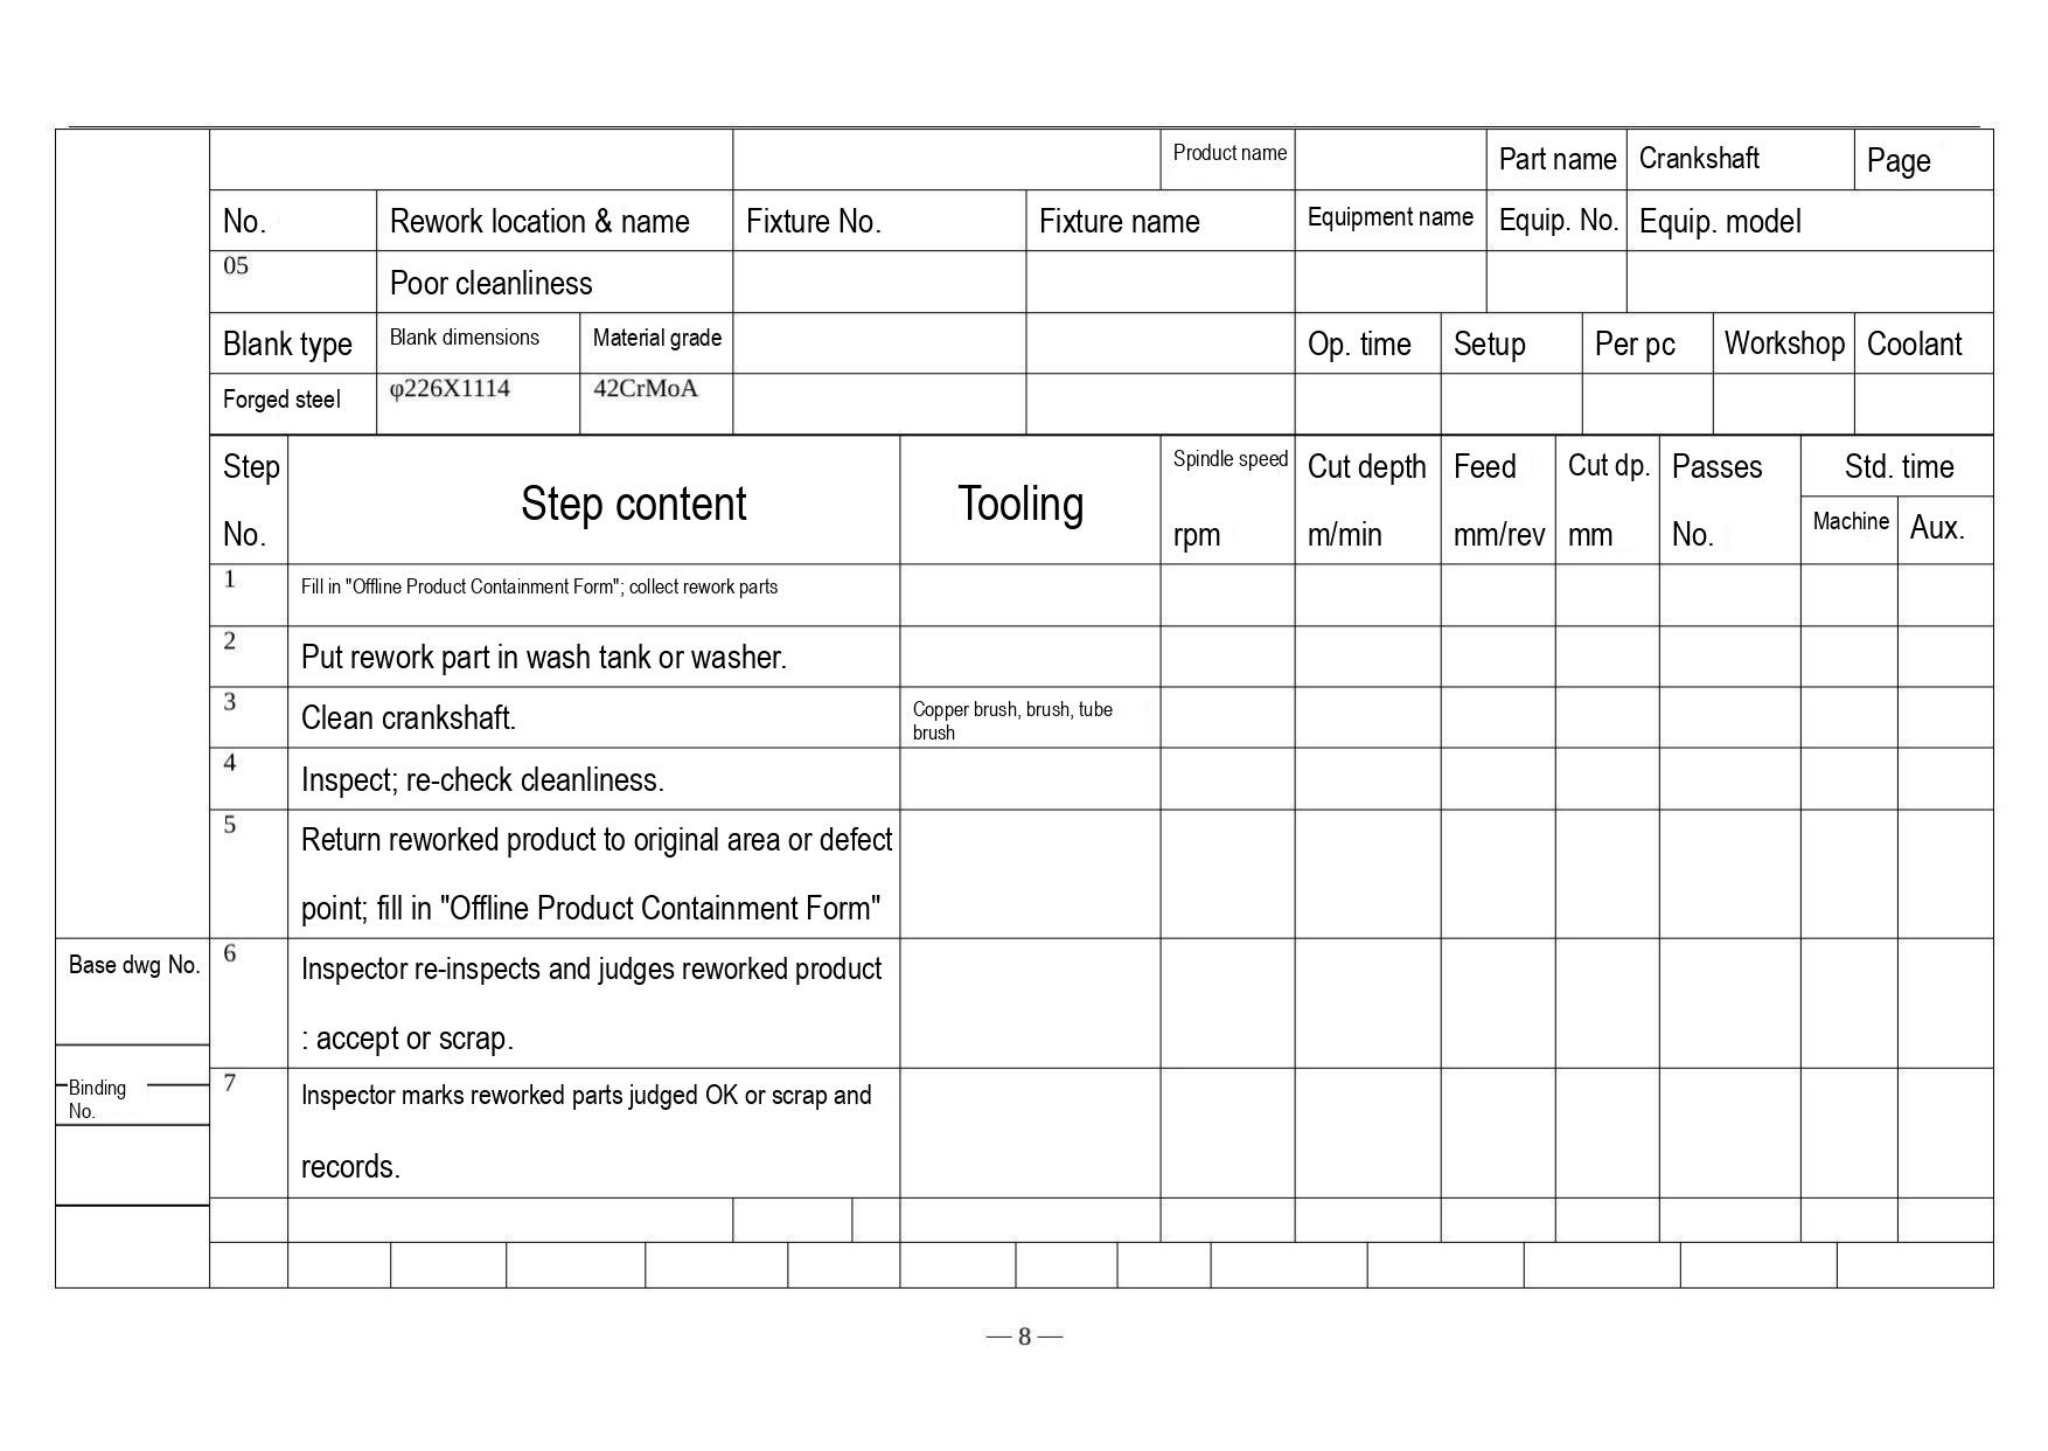| | | Product name | | Part name | Crankshaft | Page |
|---|---|---|---|---|---|---|

| No. | Rework location & name | Fixture No. | Fixture name | Equipment name | Equip. No. | Equip. model |
|---|---|---|---|---|---|---|
| 05 | Poor cleanliness | | | | | |

| Blank type | Blank dimensions | Material grade | | | Op. time | Setup | Per pc | Workshop | Coolant |
|---|---|---|---|---|---|---|---|---|---|
| Forged steel | φ226X1114 | 42CrMoA | | | | | | | |

| Step No. | Step content | Tooling | Spindle speed rpm | Cut depth m/min | Feed mm/rev | Cut dp. mm | Passes No. | Std. time Machine | Std. time Aux. |
|---|---|---|---|---|---|---|---|---|---|
| 1 | Fill in "Offline Product Containment Form"; collect rework parts | | | | | | | | |
| 2 | Put rework part in wash tank or washer. | | | | | | | | |
| 3 | Clean crankshaft. | Copper brush, brush, tube brush | | | | | | | |
| 4 | Inspect; re-check cleanliness. | | | | | | | | |
| 5 | Return reworked product to original area or defect point; fill in "Offline Product Containment Form" | | | | | | | | |
| 6 | Inspector re-inspects and judges reworked product : accept or scrap. | | | | | | | | |
| 7 | Inspector marks reworked parts judged OK or scrap and records. | | | | | | | | |

Base dwg No.

Binding No.

— 8 —
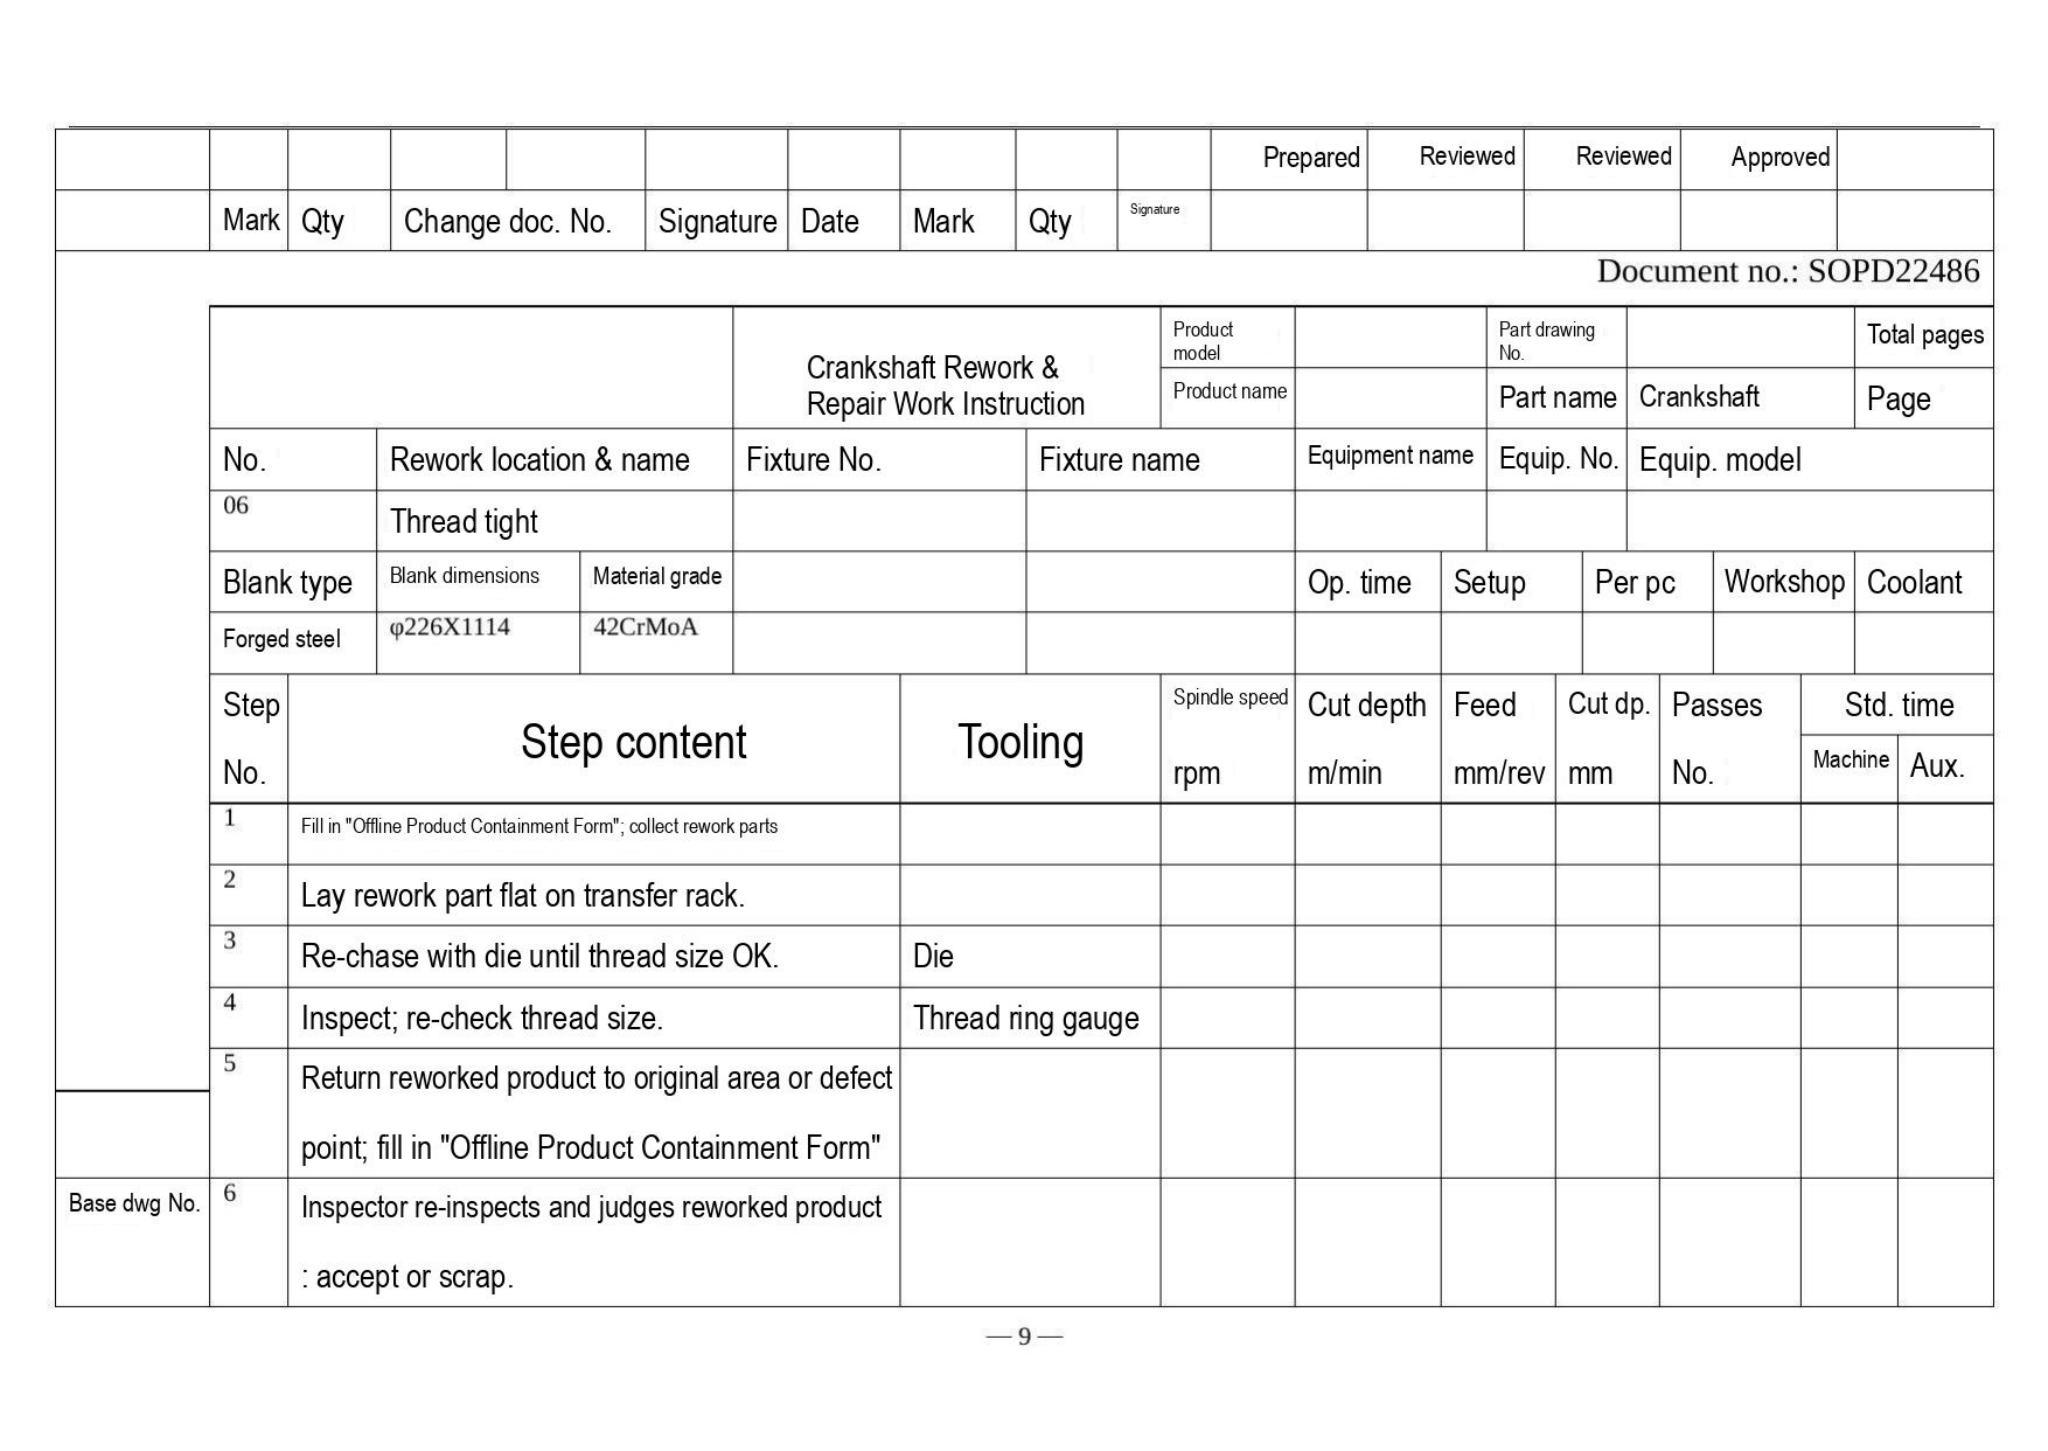Prepared | Reviewed | Reviewed | Approved

| Mark | Qty | Change doc. No. | Signature | Date | Mark | Qty | Signature |
|---|---|---|---|---|---|---|---|

Document no.: SOPD22486

| Crankshaft Rework & Repair Work Instruction | Product model | | Part drawing No. | | Total pages |
|---|---|---|---|---|---|
| | Product name | | Part name | Crankshaft | Page |

| No. | Rework location & name | Fixture No. | Fixture name | Equipment name | Equip. No. | Equip. model |
|---|---|---|---|---|---|---|
| 06 | Thread tight | | | | | |

| Blank type | Blank dimensions | Material grade | | | Op. time | Setup | Per pc | Workshop | Coolant |
|---|---|---|---|---|---|---|---|---|---|
| Forged steel | φ226X1114 | 42CrMoA | | | | | | | |

| Step No. | Step content | Tooling | Spindle speed rpm | Cut depth m/min | Feed mm/rev | Cut dp. mm | Passes No. | Std. time Machine | Std. time Aux. |
|---|---|---|---|---|---|---|---|---|---|
| 1 | Fill in "Offline Product Containment Form"; collect rework parts | | | | | | | | |
| 2 | Lay rework part flat on transfer rack. | | | | | | | | |
| 3 | Re-chase with die until thread size OK. | Die | | | | | | | |
| 4 | Inspect; re-check thread size. | Thread ring gauge | | | | | | | |
| 5 | Return reworked product to original area or defect point; fill in "Offline Product Containment Form" | | | | | | | | |
| 6 | Inspector re-inspects and judges reworked product : accept or scrap. | | | | | | | | |

Base dwg No.

— 9 —
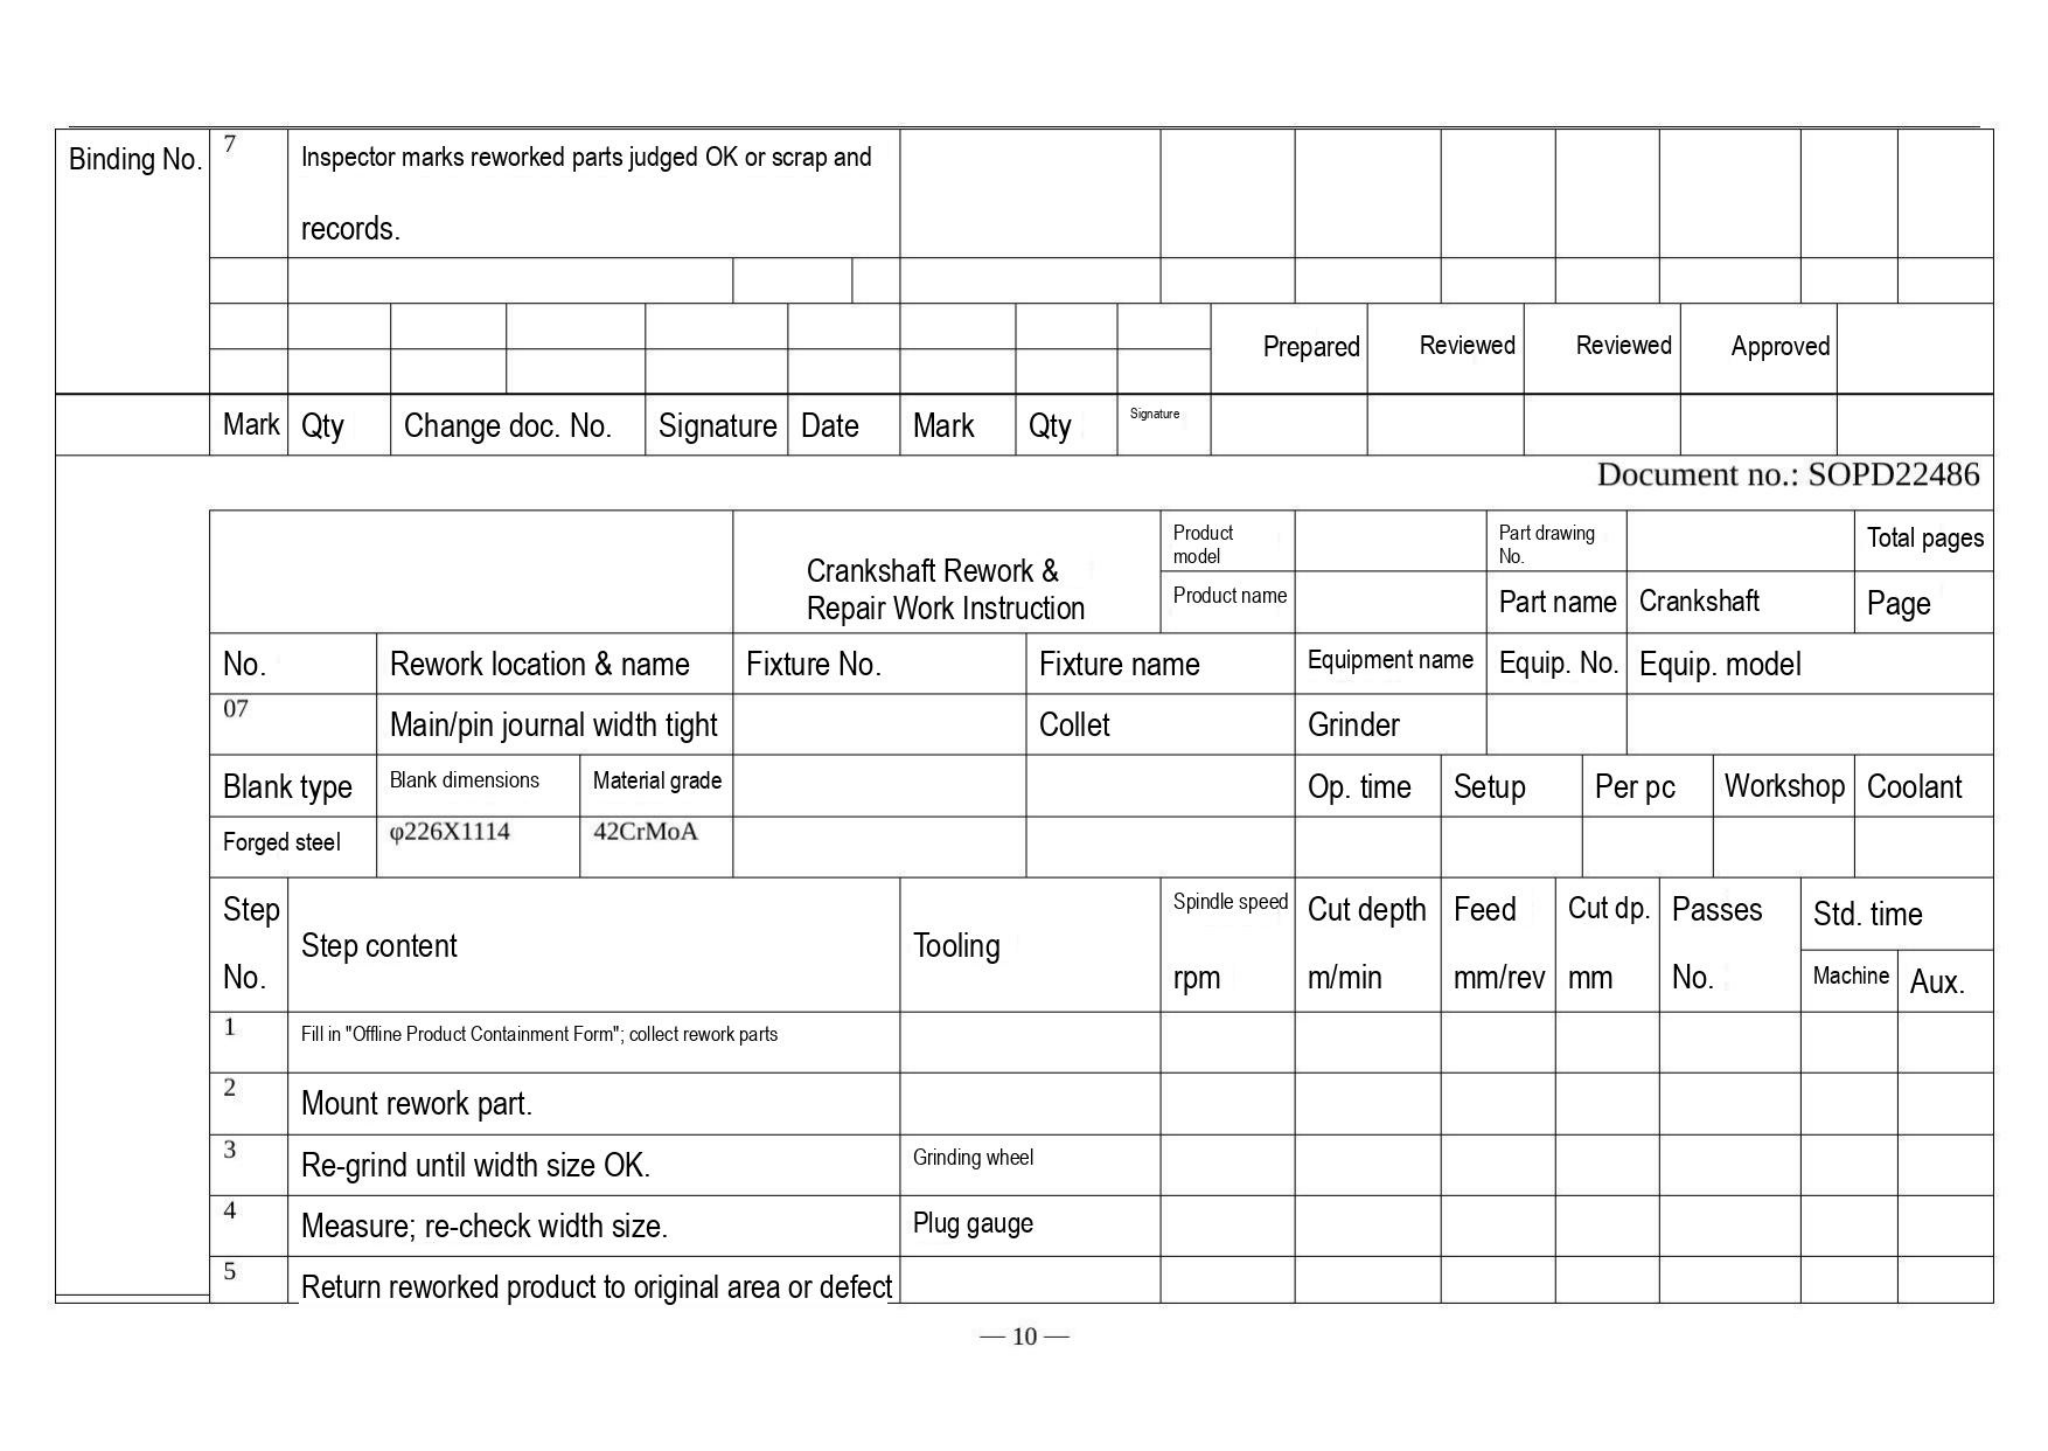| Binding No. | 7 | Inspector marks reworked parts judged OK or scrap and records. | | | | | | | |
|---|---|---|---|---|---|---|---|---|---|
| | | | | | | | | | |
| | | | | | | Prepared | Reviewed | Reviewed | Approved |
| | Mark | Qty | Change doc. No. | Signature | Date | Mark | Qty | Signature | |

Document no.: SOPD22486

| | Crankshaft Rework & Repair Work Instruction | Product model | | Part drawing No. | | Total pages |
|---|---|---|---|---|---|---|
| | | Product name | | Part name | Crankshaft | Page |

| No. | Rework location & name | Fixture No. | Fixture name | Equipment name | Equip. No. | Equip. model |
|---|---|---|---|---|---|---|
| 07 | Main/pin journal width tight | | Collet | Grinder | | |

| Blank type | Blank dimensions | Material grade | | | Op. time | Setup | Per pc | Workshop | Coolant |
|---|---|---|---|---|---|---|---|---|---|
| Forged steel | φ226X1114 | 42CrMoA | | | | | | | |

| Step No. | Step content | Tooling | Spindle speed rpm | Cut depth m/min | Feed mm/rev | Cut dp. mm | Passes No. | Std. time Machine | Std. time Aux. |
|---|---|---|---|---|---|---|---|---|---|
| 1 | Fill in "Offline Product Containment Form"; collect rework parts | | | | | | | | |
| 2 | Mount rework part. | | | | | | | | |
| 3 | Re-grind until width size OK. | Grinding wheel | | | | | | | |
| 4 | Measure; re-check width size. | Plug gauge | | | | | | | |
| 5 | Return reworked product to original area or defect | | | | | | | | |

— 10 —
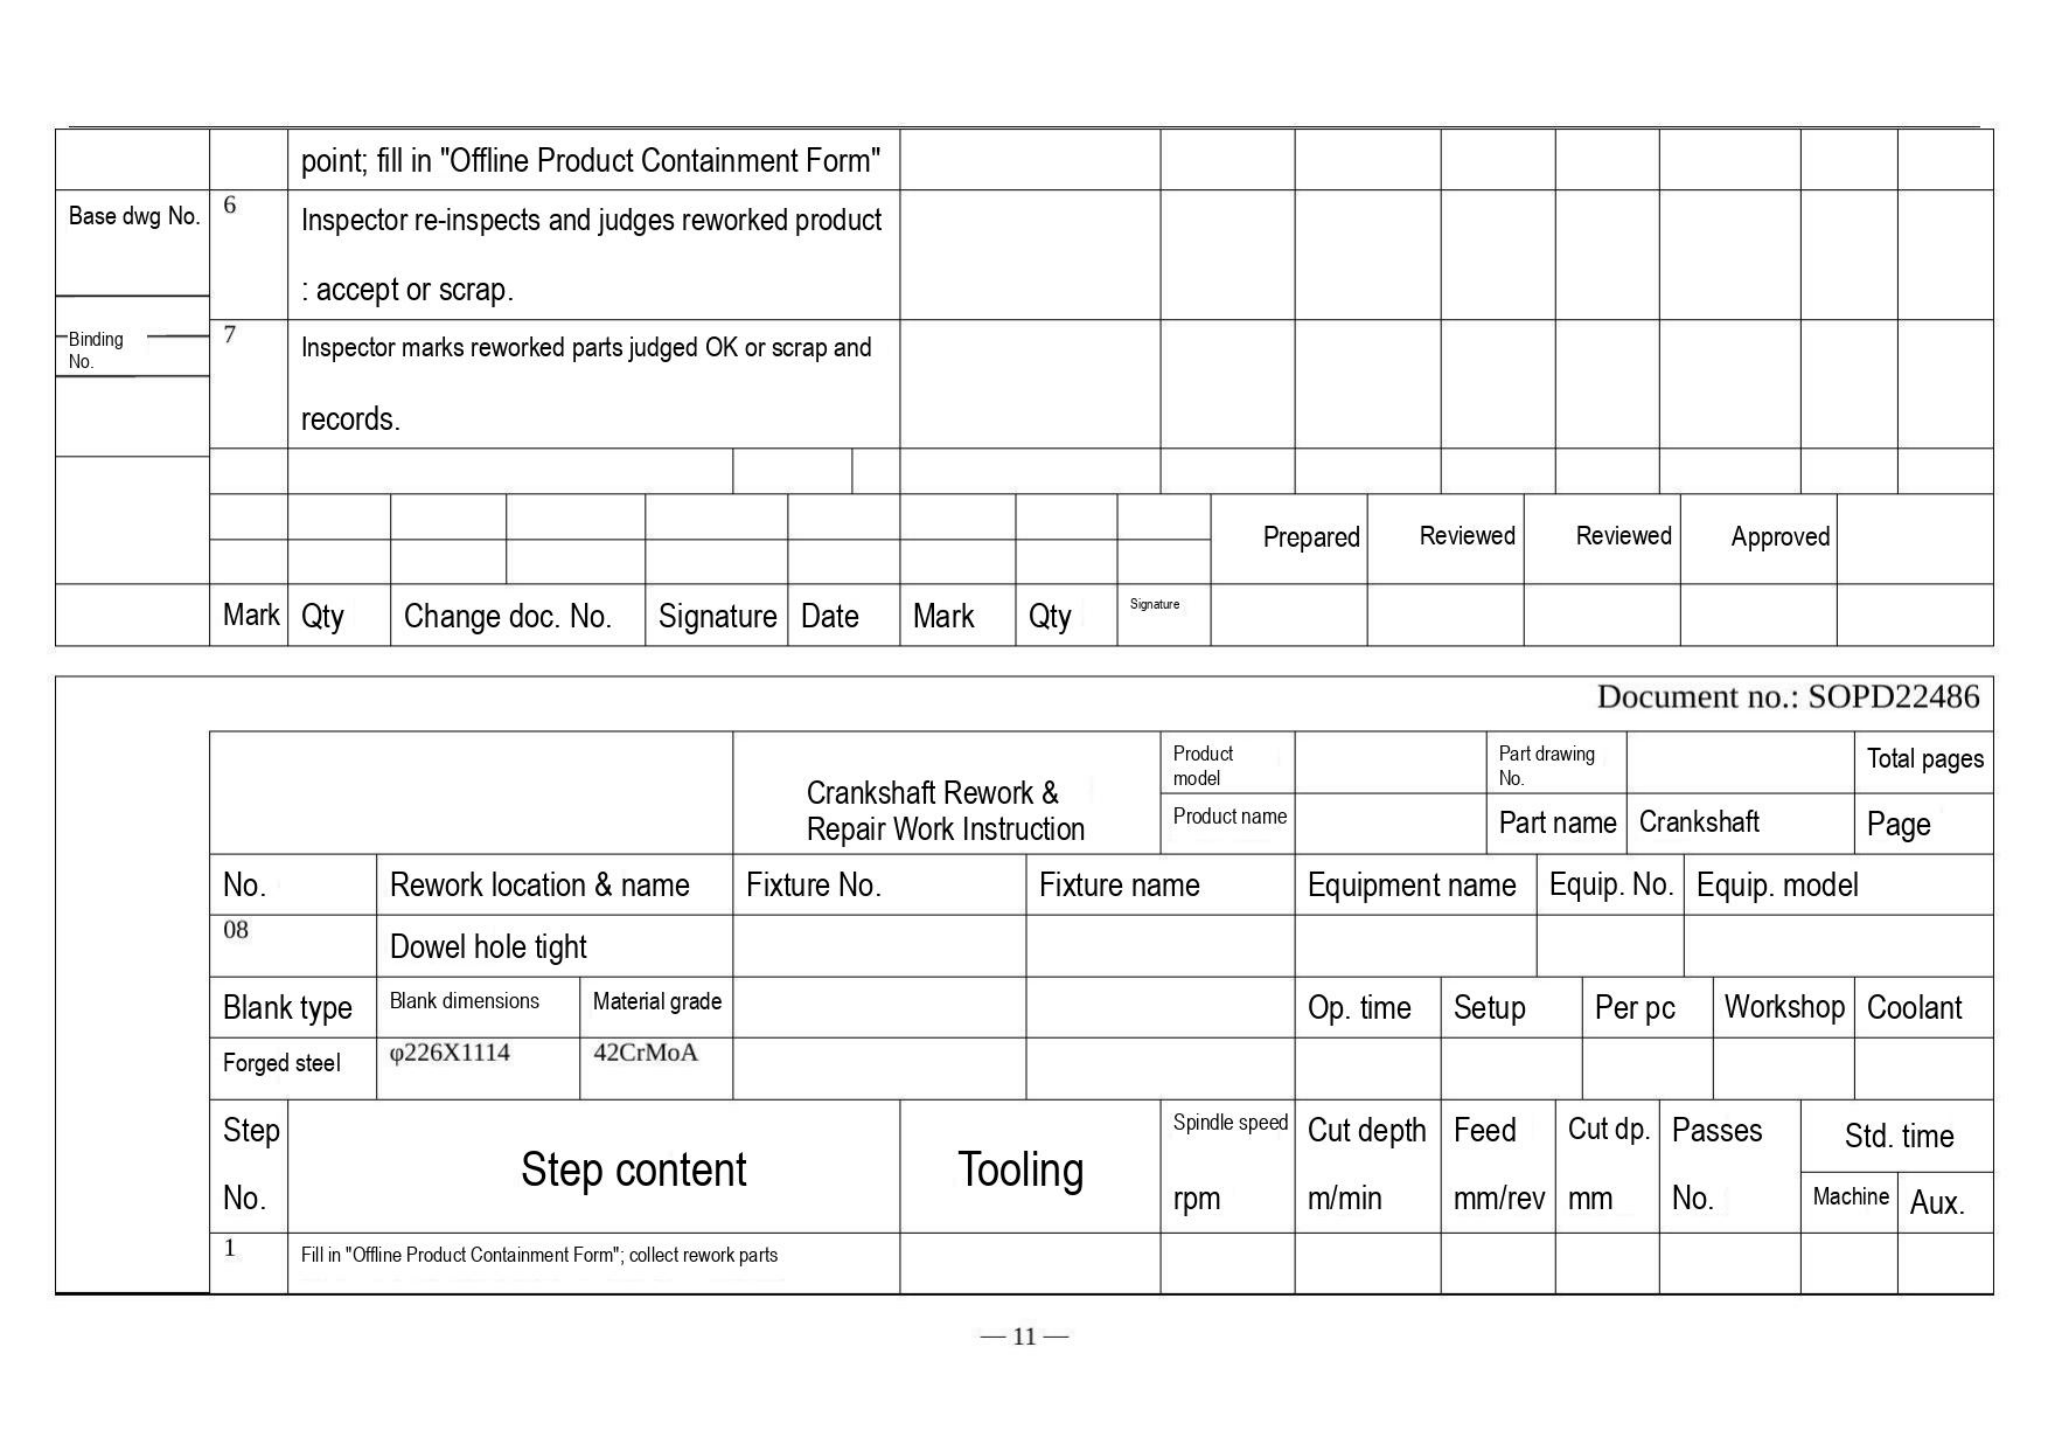| | | | | | | | | | | |
|---|---|---|---|---|---|---|---|---|---|---|
| | | point; fill in "Offline Product Containment Form" | | | | | | | | |
| Base dwg No. | 6 | Inspector re-inspects and judges reworked product : accept or scrap. | | | | | | | | |
| Binding No. | 7 | Inspector marks reworked parts judged OK or scrap and records. | | | | | | | | |

| | | | | | | | | Prepared | Reviewed | Reviewed | Approved | |
|---|---|---|---|---|---|---|---|---|---|---|---|---|
| Mark | Qty | Change doc. No. | Signature | Date | Mark | Qty | Signature | | | | | |

Document no.: SOPD22486

| | Crankshaft Rework & Repair Work Instruction | Product model | | Part drawing No. | | Total pages |
|---|---|---|---|---|---|---|
| | | Product name | | Part name | Crankshaft | Page |

| No. | Rework location & name | Fixture No. | Fixture name | Equipment name | Equip. No. | Equip. model |
|---|---|---|---|---|---|---|
| 08 | Dowel hole tight | | | | | |

| Blank type | Blank dimensions | Material grade | | | Op. time | Setup | Per pc | Workshop | Coolant |
|---|---|---|---|---|---|---|---|---|---|
| Forged steel | φ226X1114 | 42CrMoA | | | | | | | |

| Step No. | Step content | Tooling | Spindle speed rpm | Cut depth m/min | Feed mm/rev | Cut dp. mm | Passes No. | Std. time Machine | Std. time Aux. |
|---|---|---|---|---|---|---|---|---|---|
| 1 | Fill in "Offline Product Containment Form"; collect rework parts | | | | | | | | |

— 11 —
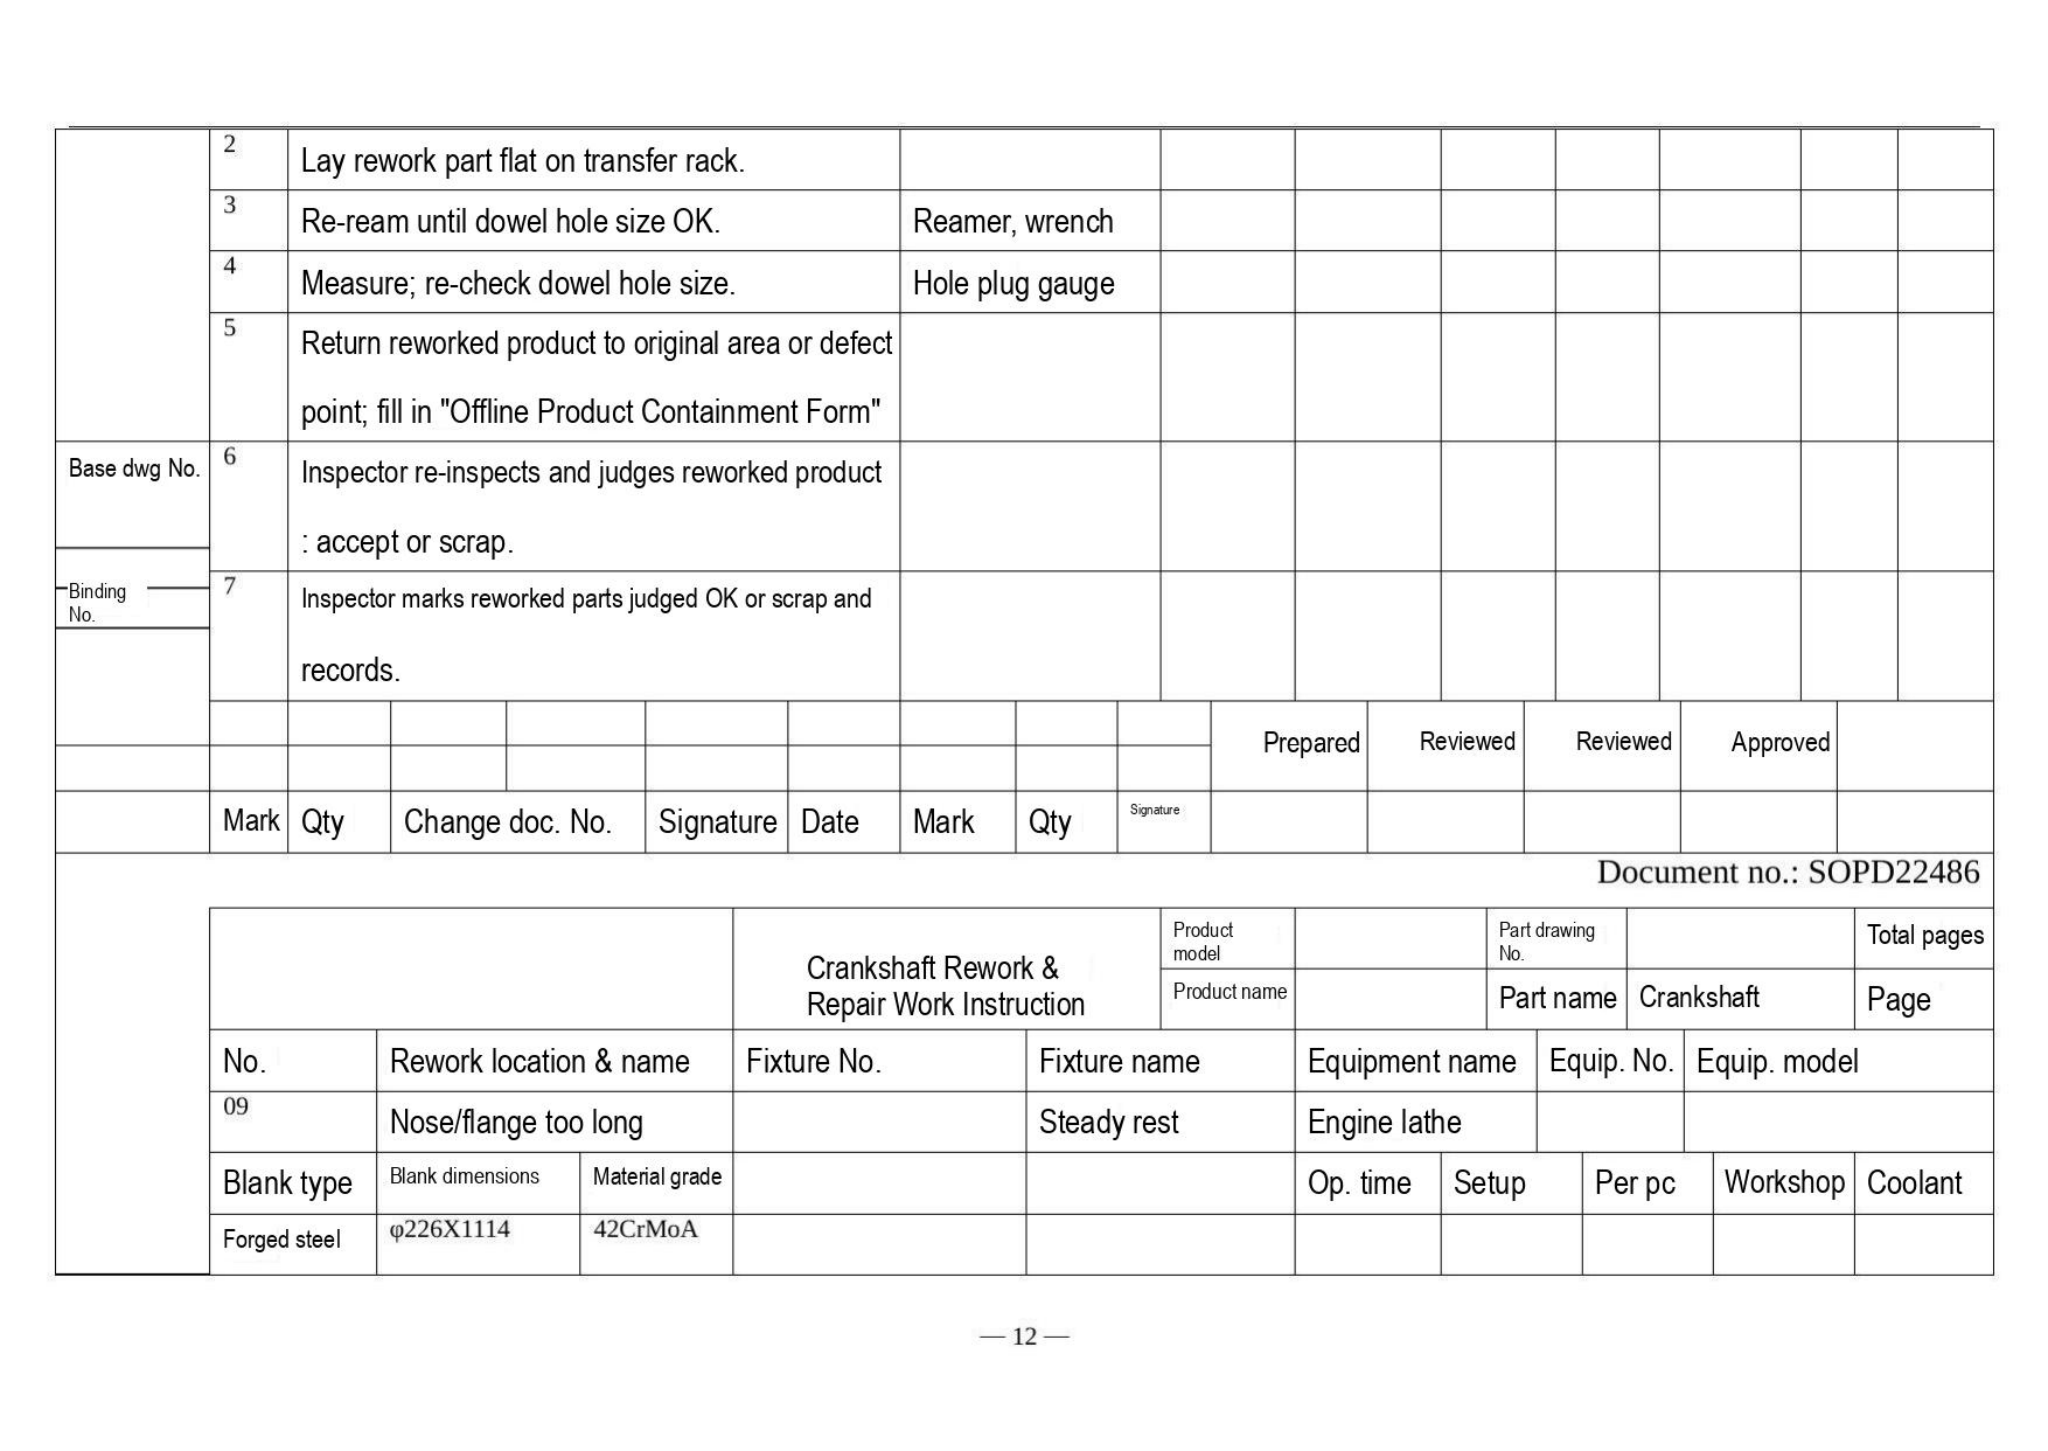| | | | |
|---|---|---|---|
| | 2 | Lay rework part flat on transfer rack. | |
| | 3 | Re-ream until dowel hole size OK. | Reamer, wrench |
| | 4 | Measure; re-check dowel hole size. | Hole plug gauge |
| | 5 | Return reworked product to original area or defect point; fill in "Offline Product Containment Form" | |
| Base dwg No. | 6 | Inspector re-inspects and judges reworked product : accept or scrap. | |
| Binding No. | 7 | Inspector marks reworked parts judged OK or scrap and records. | |

| | | | | | | | | Prepared | Reviewed | Reviewed | Approved | |
|---|---|---|---|---|---|---|---|---|---|---|---|---|
| Mark | Qty | Change doc. No. | Signature | Date | Mark | Qty | Signature | | | | | |

Document no.: SOPD22486

| | Crankshaft Rework & Repair Work Instruction | Product model | | Part drawing No. | | Total pages |
|---|---|---|---|---|---|---|
| | | Product name | | Part name | Crankshaft | Page |

| No. | Rework location & name | Fixture No. | Fixture name | Equipment name | Equip. No. | Equip. model |
|---|---|---|---|---|---|---|
| 09 | Nose/flange too long | | Steady rest | Engine lathe | | |

| Blank type | Blank dimensions | Material grade | | | Op. time | Setup | Per pc | Workshop | Coolant |
|---|---|---|---|---|---|---|---|---|---|
| Forged steel | φ226X1114 | 42CrMoA | | | | | | | |

— 12 —
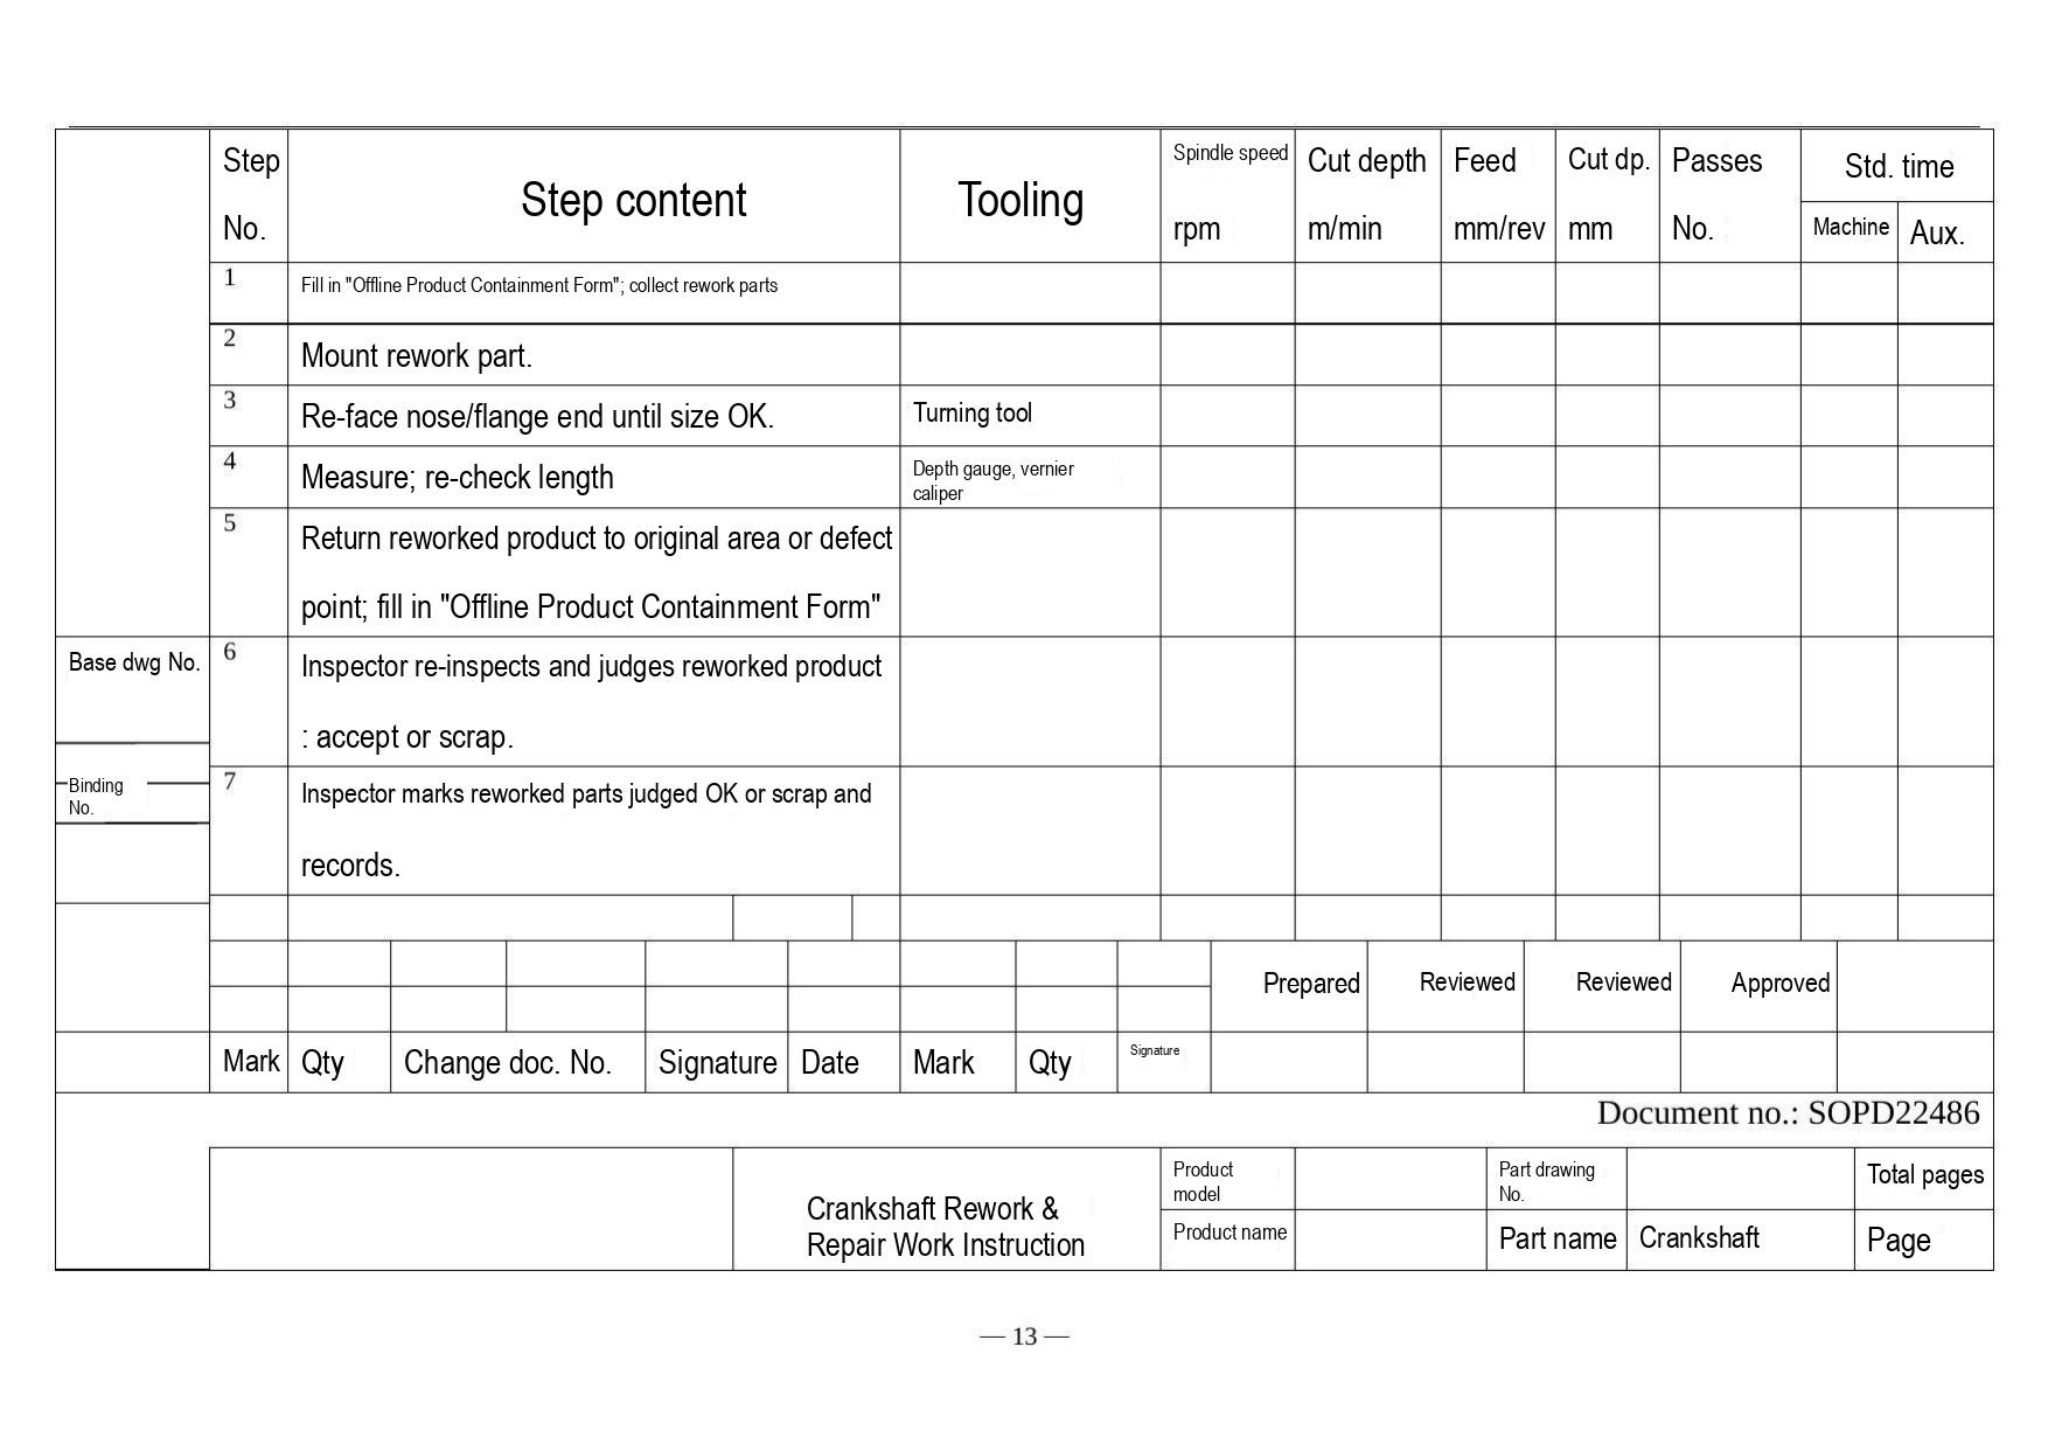| Step No. | Step content | Tooling | Spindle speed rpm | Cut depth m/min | Feed mm/rev | Cut dp. mm | Passes No. | Std. time Machine | Std. time Aux. |
|---|---|---|---|---|---|---|---|---|---|
| 1 | Fill in "Offline Product Containment Form"; collect rework parts | | | | | | | | |
| 2 | Mount rework part. | | | | | | | | |
| 3 | Re-face nose/flange end until size OK. | Turning tool | | | | | | | |
| 4 | Measure; re-check length | Depth gauge, vernier caliper | | | | | | | |
| 5 | Return reworked product to original area or defect point; fill in "Offline Product Containment Form" | | | | | | | | |
| 6 | Inspector re-inspects and judges reworked product : accept or scrap. | | | | | | | | |
| 7 | Inspector marks reworked parts judged OK or scrap and records. | | | | | | | | |

Base dwg No.

Binding No.

| Mark | Qty | Change doc. No. | Signature | Date | Mark | Qty | Signature | Prepared | Reviewed | Reviewed | Approved |
|---|---|---|---|---|---|---|---|---|---|---|---|

Document no.: SOPD22486

| Crankshaft Rework & Repair Work Instruction | Product model | | Part drawing No. | | Total pages |
|---|---|---|---|---|---|
| | Product name | | Part name | Crankshaft | Page |

— 13 —
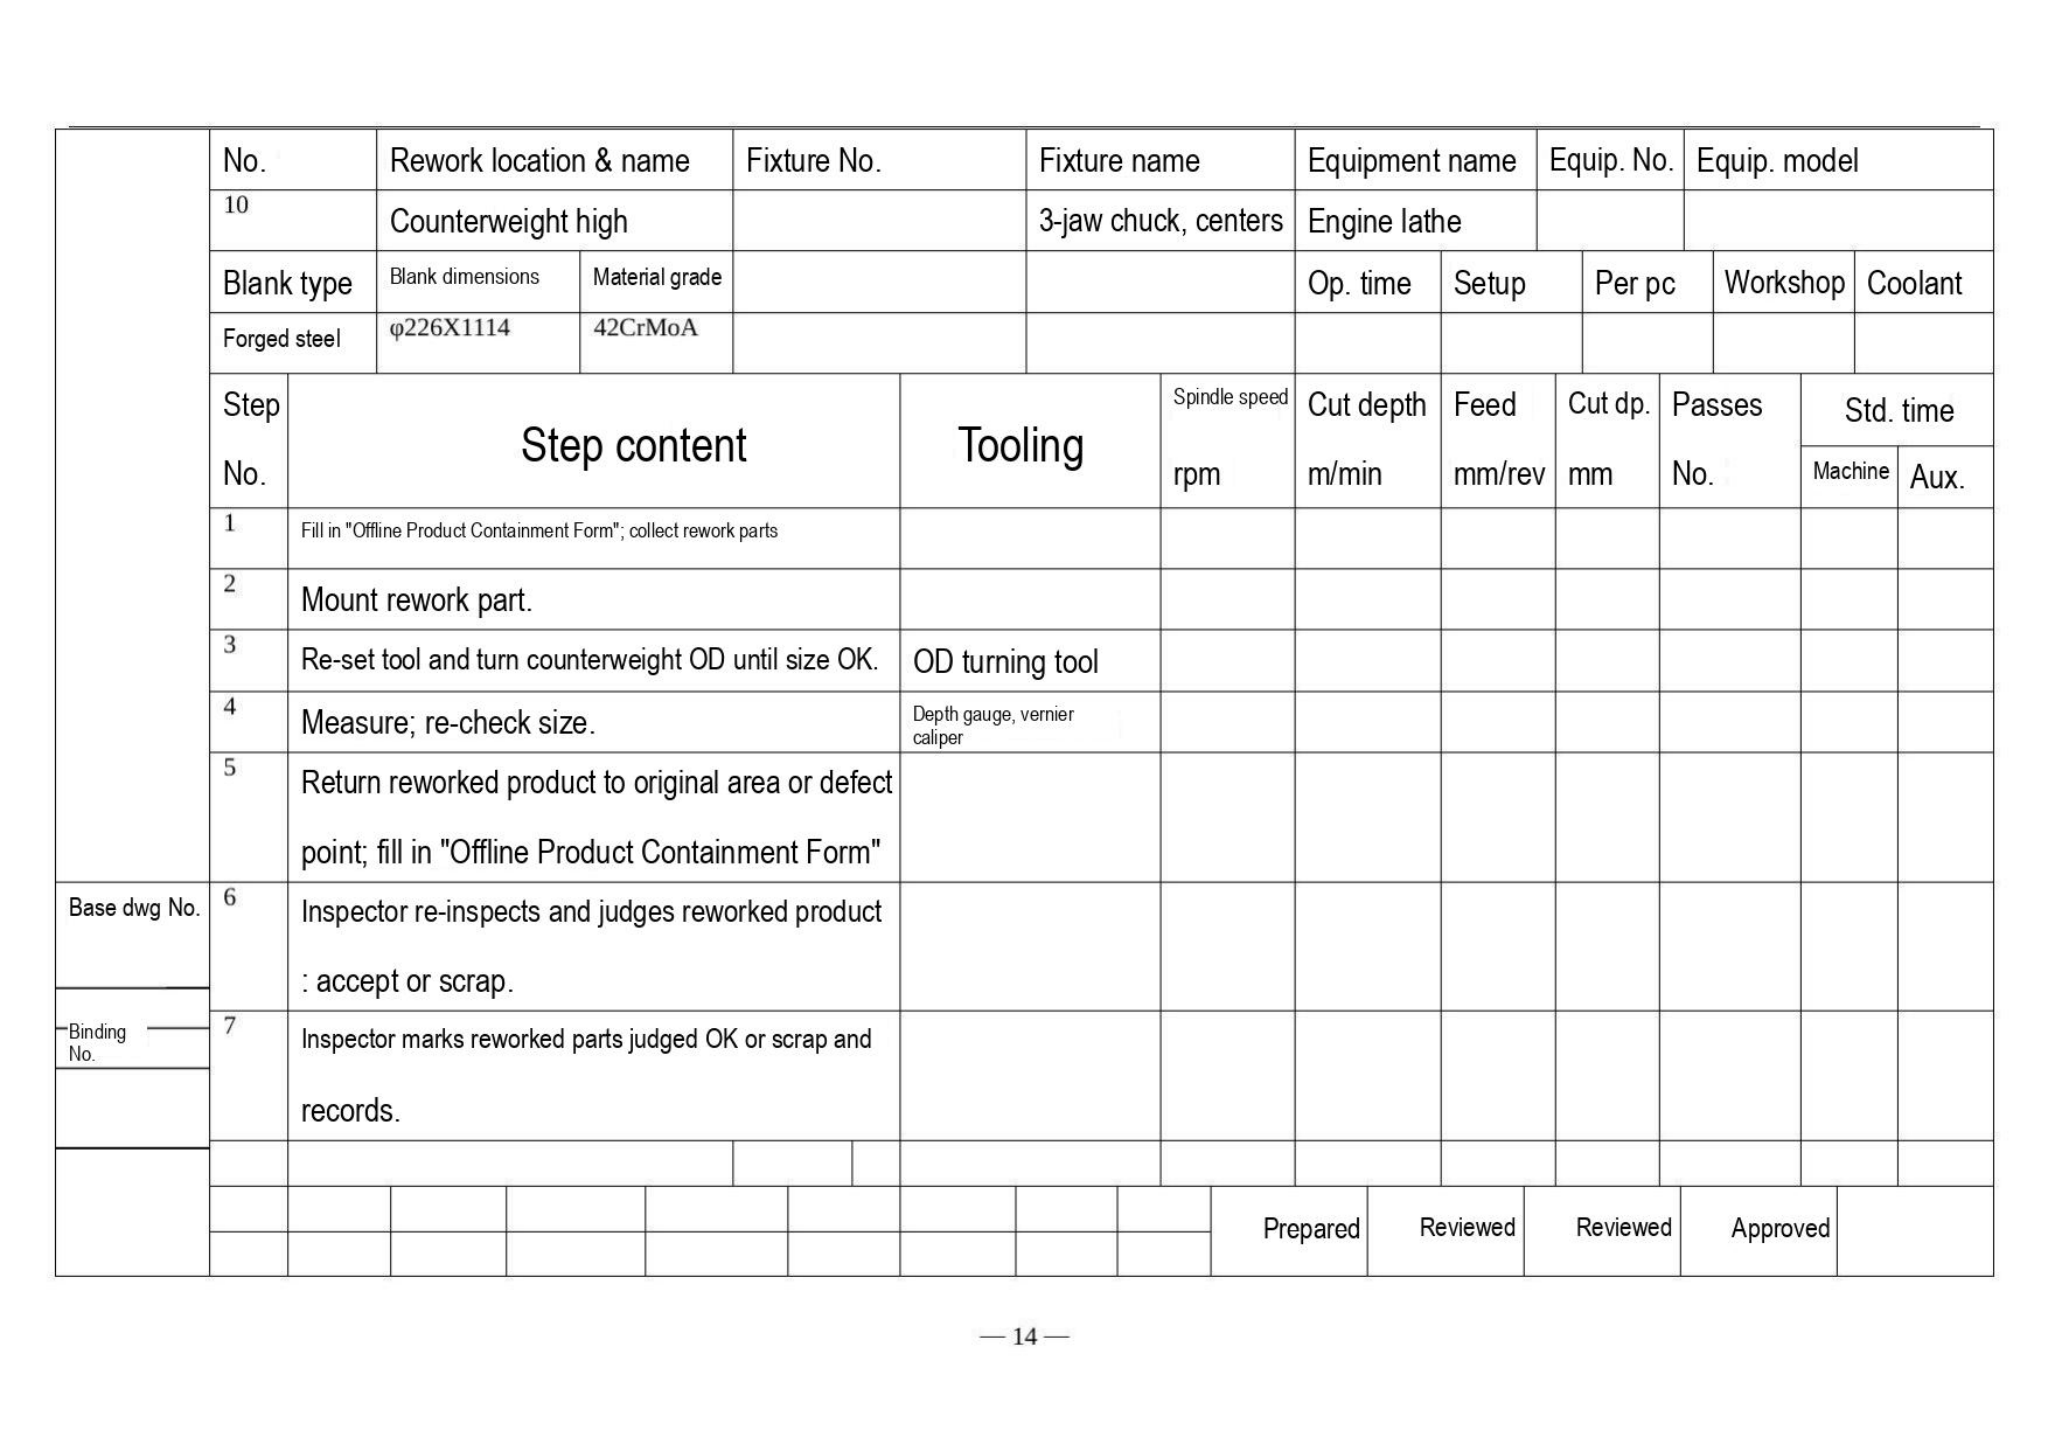| No. | Rework location & name | Fixture No. | Fixture name | Equipment name | Equip. No. | Equip. model |
|---|---|---|---|---|---|---|
| 10 | Counterweight high | | 3-jaw chuck, centers | Engine lathe | | |

| Blank type | Blank dimensions | Material grade | | | Op. time | Setup | Per pc | Workshop | Coolant |
|---|---|---|---|---|---|---|---|---|---|
| Forged steel | φ226X1114 | 42CrMoA | | | | | | | |

| Step No. | Step content | Tooling | Spindle speed rpm | Cut depth m/min | Feed mm/rev | Cut dp. mm | Passes No. | Std. time Machine | Std. time Aux. |
|---|---|---|---|---|---|---|---|---|---|
| 1 | Fill in "Offline Product Containment Form"; collect rework parts | | | | | | | | |
| 2 | Mount rework part. | | | | | | | | |
| 3 | Re-set tool and turn counterweight OD until size OK. | OD turning tool | | | | | | | |
| 4 | Measure; re-check size. | Depth gauge, vernier caliper | | | | | | | |
| 5 | Return reworked product to original area or defect point; fill in "Offline Product Containment Form" | | | | | | | | |
| 6 | Inspector re-inspects and judges reworked product : accept or scrap. | | | | | | | | |
| 7 | Inspector marks reworked parts judged OK or scrap and records. | | | | | | | | |

Base dwg No.

Binding No.

| Prepared | Reviewed | Reviewed | Approved |
|---|---|---|---|
| | | | |

— 14 —